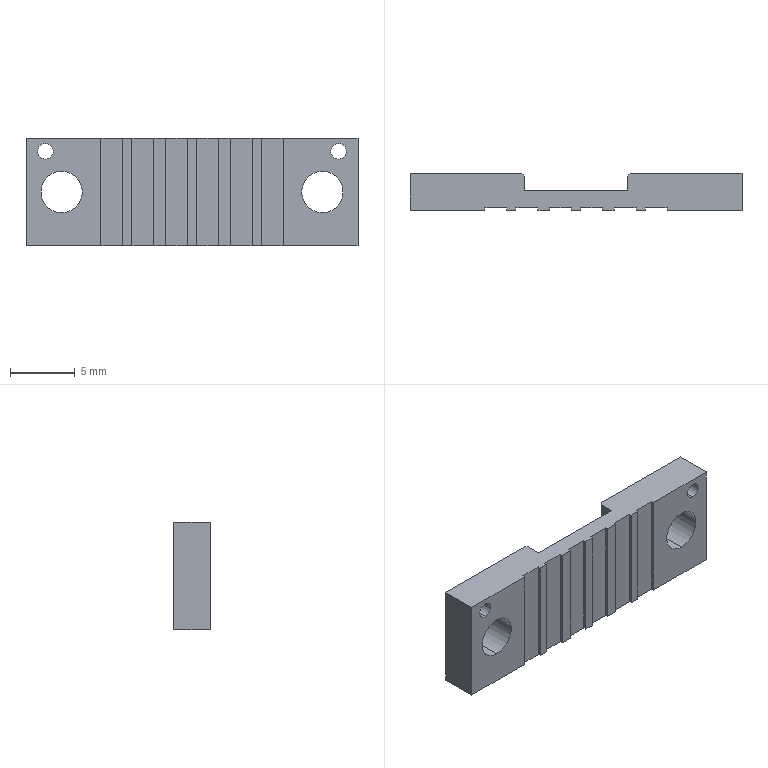Part | SolidWorks | features ICE 3, Chamfer 1, Extrusion 1 | 1 solid | 44 faces | box 25.7 x 2.85 x 8.3 mm | volume 448.741 mm3 | plane 36 | cylinder 8 | commonest cylinder face diameters 1.2 x4 3.2 x4
STEP:
#1=CARTESIAN_POINT('',(11.35,0.,2.55));
#2=VERTEX_POINT('',#1);
#3=CARTESIAN_POINT('',(11.35,0.,3.75));
#4=VERTEX_POINT('',#3);
#5=CARTESIAN_POINT('',(11.35,0.,3.15));
#6=DIRECTION('',(0.,1.,0.));
#7=DIRECTION('',(0.,0.,-1.));
#8=AXIS2_PLACEMENT_3D('',#5,#6,#7);
#9=CIRCLE('',#8,0.6);
#10=EDGE_CURVE('',#2,#4,#9,.T.);
#11=ORIENTED_EDGE('',*,*,#10,.F.);
#12=CARTESIAN_POINT('',(11.35,2.85,2.55));
#13=VERTEX_POINT('',#12);
#14=CARTESIAN_POINT('',(11.35,0.,2.55));
#15=DIRECTION('',(0.,1.,0.));
#16=VECTOR('',#15,1000.);
#17=LINE('',#14,#16);
#18=EDGE_CURVE('',#2,#13,#17,.T.);
#19=ORIENTED_EDGE('',*,*,#18,.T.);
#20=CARTESIAN_POINT('',(11.35,2.85,3.75));
#21=VERTEX_POINT('',#20);
#22=CARTESIAN_POINT('',(11.35,2.85,3.15));
#23=DIRECTION('',(0.,1.,0.));
#24=DIRECTION('',(0.,0.,-1.));
#25=AXIS2_PLACEMENT_3D('',#22,#23,#24);
#26=CIRCLE('',#25,0.6);
#27=EDGE_CURVE('',#13,#21,#26,.T.);
#28=ORIENTED_EDGE('',*,*,#27,.T.);
#29=CARTESIAN_POINT('',(11.35,0.,3.75));
#30=DIRECTION('',(0.,1.,0.));
#31=VECTOR('',#30,1000.);
#32=LINE('',#29,#31);
#33=EDGE_CURVE('',#4,#21,#32,.T.);
#34=ORIENTED_EDGE('',*,*,#33,.F.);
#35=EDGE_LOOP('',(#11,#19,#28,#34));
#36=FACE_OUTER_BOUND('',#35,.T.);
#37=CARTESIAN_POINT('',(11.35,0.,3.15));
#38=DIRECTION('',(0.,1.,0.));
#39=DIRECTION('',(0.,0.,1.));
#40=AXIS2_PLACEMENT_3D('',#37,#38,#39);
#41=CYLINDRICAL_SURFACE('',#40,0.6);
#42=ADVANCED_FACE('',(#36),#41,.F.);
#43=CARTESIAN_POINT('',(10.1,0.,-1.6));
#44=VERTEX_POINT('',#43);
#45=CARTESIAN_POINT('',(10.1,0.,1.6));
#46=VERTEX_POINT('',#45);
#47=CARTESIAN_POINT('',(10.1,0.,0.));
#48=DIRECTION('',(0.,1.,0.));
#49=DIRECTION('',(0.,0.,-1.));
#50=AXIS2_PLACEMENT_3D('',#47,#48,#49);
#51=CIRCLE('',#50,1.6);
#52=EDGE_CURVE('',#44,#46,#51,.T.);
#53=ORIENTED_EDGE('',*,*,#52,.F.);
#54=CARTESIAN_POINT('',(10.1,2.85,-1.6));
#55=VERTEX_POINT('',#54);
#56=CARTESIAN_POINT('',(10.1,0.,-1.6));
#57=DIRECTION('',(0.,1.,0.));
#58=VECTOR('',#57,1000.);
#59=LINE('',#56,#58);
#60=EDGE_CURVE('',#44,#55,#59,.T.);
#61=ORIENTED_EDGE('',*,*,#60,.T.);
#62=CARTESIAN_POINT('',(10.1,2.85,1.6));
#63=VERTEX_POINT('',#62);
#64=CARTESIAN_POINT('',(10.1,2.85,0.));
#65=DIRECTION('',(0.,1.,0.));
#66=DIRECTION('',(0.,0.,-1.));
#67=AXIS2_PLACEMENT_3D('',#64,#65,#66);
#68=CIRCLE('',#67,1.6);
#69=EDGE_CURVE('',#55,#63,#68,.T.);
#70=ORIENTED_EDGE('',*,*,#69,.T.);
#71=CARTESIAN_POINT('',(10.1,0.,1.6));
#72=DIRECTION('',(0.,1.,0.));
#73=VECTOR('',#72,1000.);
#74=LINE('',#71,#73);
#75=EDGE_CURVE('',#46,#63,#74,.T.);
#76=ORIENTED_EDGE('',*,*,#75,.F.);
#77=EDGE_LOOP('',(#53,#61,#70,#76));
#78=FACE_OUTER_BOUND('',#77,.T.);
#79=CARTESIAN_POINT('',(10.1,0.,0.));
#80=DIRECTION('',(0.,1.,0.));
#81=DIRECTION('',(0.,0.,1.));
#82=AXIS2_PLACEMENT_3D('',#79,#80,#81);
#83=CYLINDRICAL_SURFACE('',#82,1.6);
#84=ADVANCED_FACE('',(#78),#83,.F.);
#85=CARTESIAN_POINT('',(-11.35,0.,2.55));
#86=VERTEX_POINT('',#85);
#87=CARTESIAN_POINT('',(-11.35,0.,3.75));
#88=VERTEX_POINT('',#87);
#89=CARTESIAN_POINT('',(-11.35,0.,3.15));
#90=DIRECTION('',(0.,1.,0.));
#91=DIRECTION('',(0.,0.,1.));
#92=AXIS2_PLACEMENT_3D('',#89,#90,#91);
#93=CIRCLE('',#92,0.6);
#94=EDGE_CURVE('',#86,#88,#93,.T.);
#95=ORIENTED_EDGE('',*,*,#94,.F.);
#96=CARTESIAN_POINT('',(-11.35,2.85,2.55));
#97=VERTEX_POINT('',#96);
#98=CARTESIAN_POINT('',(-11.35,0.,2.55));
#99=DIRECTION('',(0.,1.,0.));
#100=VECTOR('',#99,1000.);
#101=LINE('',#98,#100);
#102=EDGE_CURVE('',#86,#97,#101,.T.);
#103=ORIENTED_EDGE('',*,*,#102,.T.);
#104=CARTESIAN_POINT('',(-11.35,2.85,3.75));
#105=VERTEX_POINT('',#104);
#106=CARTESIAN_POINT('',(-11.35,2.85,3.15));
#107=DIRECTION('',(0.,1.,0.));
#108=DIRECTION('',(0.,0.,1.));
#109=AXIS2_PLACEMENT_3D('',#106,#107,#108);
#110=CIRCLE('',#109,0.6);
#111=EDGE_CURVE('',#97,#105,#110,.T.);
#112=ORIENTED_EDGE('',*,*,#111,.T.);
#113=CARTESIAN_POINT('',(-11.35,0.,3.75));
#114=DIRECTION('',(0.,1.,0.));
#115=VECTOR('',#114,1000.);
#116=LINE('',#113,#115);
#117=EDGE_CURVE('',#88,#105,#116,.T.);
#118=ORIENTED_EDGE('',*,*,#117,.F.);
#119=EDGE_LOOP('',(#95,#103,#112,#118));
#120=FACE_OUTER_BOUND('',#119,.T.);
#121=CARTESIAN_POINT('',(-11.35,0.,3.15));
#122=DIRECTION('',(0.,1.,0.));
#123=DIRECTION('',(0.,0.,1.));
#124=AXIS2_PLACEMENT_3D('',#121,#122,#123);
#125=CYLINDRICAL_SURFACE('',#124,0.6);
#126=ADVANCED_FACE('',(#120),#125,.F.);
#127=CARTESIAN_POINT('',(-10.1,0.,-1.6));
#128=VERTEX_POINT('',#127);
#129=CARTESIAN_POINT('',(-10.1,0.,1.6));
#130=VERTEX_POINT('',#129);
#131=CARTESIAN_POINT('',(-10.1,0.,0.));
#132=DIRECTION('',(0.,1.,0.));
#133=DIRECTION('',(0.,0.,1.));
#134=AXIS2_PLACEMENT_3D('',#131,#132,#133);
#135=CIRCLE('',#134,1.6);
#136=EDGE_CURVE('',#128,#130,#135,.T.);
#137=ORIENTED_EDGE('',*,*,#136,.F.);
#138=CARTESIAN_POINT('',(-10.1,2.85,-1.6));
#139=VERTEX_POINT('',#138);
#140=CARTESIAN_POINT('',(-10.1,0.,-1.6));
#141=DIRECTION('',(0.,1.,0.));
#142=VECTOR('',#141,1000.);
#143=LINE('',#140,#142);
#144=EDGE_CURVE('',#128,#139,#143,.T.);
#145=ORIENTED_EDGE('',*,*,#144,.T.);
#146=CARTESIAN_POINT('',(-10.1,2.85,1.6));
#147=VERTEX_POINT('',#146);
#148=CARTESIAN_POINT('',(-10.1,2.85,0.));
#149=DIRECTION('',(0.,1.,0.));
#150=DIRECTION('',(0.,0.,1.));
#151=AXIS2_PLACEMENT_3D('',#148,#149,#150);
#152=CIRCLE('',#151,1.6);
#153=EDGE_CURVE('',#139,#147,#152,.T.);
#154=ORIENTED_EDGE('',*,*,#153,.T.);
#155=CARTESIAN_POINT('',(-10.1,0.,1.6));
#156=DIRECTION('',(0.,1.,0.));
#157=VECTOR('',#156,1000.);
#158=LINE('',#155,#157);
#159=EDGE_CURVE('',#130,#147,#158,.T.);
#160=ORIENTED_EDGE('',*,*,#159,.F.);
#161=EDGE_LOOP('',(#137,#145,#154,#160));
#162=FACE_OUTER_BOUND('',#161,.T.);
#163=CARTESIAN_POINT('',(-10.1,0.,0.));
#164=DIRECTION('',(0.,1.,0.));
#165=DIRECTION('',(0.,0.,1.));
#166=AXIS2_PLACEMENT_3D('',#163,#164,#165);
#167=CYLINDRICAL_SURFACE('',#166,1.6);
#168=ADVANCED_FACE('',(#162),#167,.F.);
#169=CARTESIAN_POINT('',(12.85,2.85,-4.15));
#170=VERTEX_POINT('',#169);
#171=CARTESIAN_POINT('',(4.2,2.85,-4.15));
#172=VERTEX_POINT('',#171);
#173=CARTESIAN_POINT('',(-12.85,2.85,-4.15));
#174=DIRECTION('',(-1.,0.,0.));
#175=VECTOR('',#174,1000.);
#176=LINE('',#173,#175);
#177=EDGE_CURVE('',#170,#172,#176,.T.);
#178=ORIENTED_EDGE('',*,*,#177,.T.);
#179=CARTESIAN_POINT('',(4.2,2.85,4.15));
#180=VERTEX_POINT('',#179);
#181=CARTESIAN_POINT('',(4.2,2.85,4.15));
#182=DIRECTION('',(0.,0.,1.));
#183=VECTOR('',#182,1000.);
#184=LINE('',#181,#183);
#185=EDGE_CURVE('',#172,#180,#184,.T.);
#186=ORIENTED_EDGE('',*,*,#185,.T.);
#187=CARTESIAN_POINT('',(12.85,2.85,4.15));
#188=VERTEX_POINT('',#187);
#189=CARTESIAN_POINT('',(-12.85,2.85,4.15));
#190=DIRECTION('',(1.,0.,0.));
#191=VECTOR('',#190,1000.);
#192=LINE('',#189,#191);
#193=EDGE_CURVE('',#180,#188,#192,.T.);
#194=ORIENTED_EDGE('',*,*,#193,.T.);
#195=CARTESIAN_POINT('',(12.85,2.85,-4.15));
#196=DIRECTION('',(0.,0.,-1.));
#197=VECTOR('',#196,1000.);
#198=LINE('',#195,#197);
#199=EDGE_CURVE('',#188,#170,#198,.T.);
#200=ORIENTED_EDGE('',*,*,#199,.T.);
#201=EDGE_LOOP('',(#178,#186,#194,#200));
#202=FACE_OUTER_BOUND('',#201,.T.);
#203=CARTESIAN_POINT('',(10.1,2.85,0.));
#204=DIRECTION('',(0.,1.,0.));
#205=DIRECTION('',(0.,0.,-1.));
#206=AXIS2_PLACEMENT_3D('',#203,#204,#205);
#207=CIRCLE('',#206,1.6);
#208=EDGE_CURVE('',#63,#55,#207,.T.);
#209=ORIENTED_EDGE('',*,*,#208,.F.);
#210=ORIENTED_EDGE('',*,*,#69,.F.);
#211=EDGE_LOOP('',(#209,#210));
#212=FACE_BOUND('',#211,.T.);
#213=CARTESIAN_POINT('',(11.35,2.85,3.15));
#214=DIRECTION('',(0.,1.,0.));
#215=DIRECTION('',(0.,0.,-1.));
#216=AXIS2_PLACEMENT_3D('',#213,#214,#215);
#217=CIRCLE('',#216,0.6);
#218=EDGE_CURVE('',#21,#13,#217,.T.);
#219=ORIENTED_EDGE('',*,*,#218,.F.);
#220=ORIENTED_EDGE('',*,*,#27,.F.);
#221=EDGE_LOOP('',(#219,#220));
#222=FACE_BOUND('',#221,.T.);
#223=CARTESIAN_POINT('',(0.,2.85,0.));
#224=DIRECTION('',(0.,1.,0.));
#225=DIRECTION('',(0.,0.,1.));
#226=AXIS2_PLACEMENT_3D('',#223,#224,#225);
#227=PLANE('',#226);
#228=ADVANCED_FACE('',(#202,#212,#222),#227,.T.);
#229=CARTESIAN_POINT('',(10.1,0.,0.));
#230=DIRECTION('',(0.,1.,0.));
#231=DIRECTION('',(0.,0.,-1.));
#232=AXIS2_PLACEMENT_3D('',#229,#230,#231);
#233=CIRCLE('',#232,1.6);
#234=EDGE_CURVE('',#46,#44,#233,.T.);
#235=ORIENTED_EDGE('',*,*,#234,.T.);
#236=ORIENTED_EDGE('',*,*,#52,.T.);
#237=EDGE_LOOP('',(#235,#236));
#238=FACE_BOUND('',#237,.T.);
#239=CARTESIAN_POINT('',(11.35,0.,3.15));
#240=DIRECTION('',(0.,1.,0.));
#241=DIRECTION('',(0.,0.,-1.));
#242=AXIS2_PLACEMENT_3D('',#239,#240,#241);
#243=CIRCLE('',#242,0.6);
#244=EDGE_CURVE('',#4,#2,#243,.T.);
#245=ORIENTED_EDGE('',*,*,#244,.T.);
#246=ORIENTED_EDGE('',*,*,#10,.T.);
#247=EDGE_LOOP('',(#245,#246));
#248=FACE_BOUND('',#247,.T.);
#249=CARTESIAN_POINT('',(7.05,0.,4.15));
#250=VERTEX_POINT('',#249);
#251=CARTESIAN_POINT('',(12.85,0.,4.15));
#252=VERTEX_POINT('',#251);
#253=CARTESIAN_POINT('',(-12.85,0.,4.15));
#254=DIRECTION('',(1.,0.,0.));
#255=VECTOR('',#254,1000.);
#256=LINE('',#253,#255);
#257=EDGE_CURVE('',#250,#252,#256,.T.);
#258=ORIENTED_EDGE('',*,*,#257,.F.);
#259=CARTESIAN_POINT('',(7.05,0.,-4.15));
#260=VERTEX_POINT('',#259);
#261=CARTESIAN_POINT('',(7.05,0.,4.15));
#262=DIRECTION('',(0.,0.,1.));
#263=VECTOR('',#262,1000.);
#264=LINE('',#261,#263);
#265=EDGE_CURVE('',#260,#250,#264,.T.);
#266=ORIENTED_EDGE('',*,*,#265,.F.);
#267=CARTESIAN_POINT('',(12.85,0.,-4.15));
#268=VERTEX_POINT('',#267);
#269=CARTESIAN_POINT('',(-12.85,0.,-4.15));
#270=DIRECTION('',(-1.,0.,0.));
#271=VECTOR('',#270,1000.);
#272=LINE('',#269,#271);
#273=EDGE_CURVE('',#268,#260,#272,.T.);
#274=ORIENTED_EDGE('',*,*,#273,.F.);
#275=CARTESIAN_POINT('',(12.85,0.,-4.15));
#276=DIRECTION('',(0.,0.,-1.));
#277=VECTOR('',#276,1000.);
#278=LINE('',#275,#277);
#279=EDGE_CURVE('',#252,#268,#278,.T.);
#280=ORIENTED_EDGE('',*,*,#279,.F.);
#281=EDGE_LOOP('',(#258,#266,#274,#280));
#282=FACE_OUTER_BOUND('',#281,.T.);
#283=CARTESIAN_POINT('',(0.,0.,0.));
#284=DIRECTION('',(0.,1.,0.));
#285=DIRECTION('',(0.,0.,1.));
#286=AXIS2_PLACEMENT_3D('',#283,#284,#285);
#287=PLANE('',#286);
#288=ADVANCED_FACE('',(#238,#248,#282),#287,.F.);
#289=CARTESIAN_POINT('',(5.35,0.,-4.15));
#290=VERTEX_POINT('',#289);
#291=CARTESIAN_POINT('',(4.65,0.,-4.15));
#292=VERTEX_POINT('',#291);
#293=CARTESIAN_POINT('',(-12.85,0.,-4.15));
#294=DIRECTION('',(-1.,0.,0.));
#295=VECTOR('',#294,1000.);
#296=LINE('',#293,#295);
#297=EDGE_CURVE('',#290,#292,#296,.T.);
#298=ORIENTED_EDGE('',*,*,#297,.F.);
#299=CARTESIAN_POINT('',(5.35,0.,4.15));
#300=VERTEX_POINT('',#299);
#301=CARTESIAN_POINT('',(5.35,0.,4.15));
#302=DIRECTION('',(0.,0.,-1.));
#303=VECTOR('',#302,1000.);
#304=LINE('',#301,#303);
#305=EDGE_CURVE('',#300,#290,#304,.T.);
#306=ORIENTED_EDGE('',*,*,#305,.F.);
#307=CARTESIAN_POINT('',(4.65,0.,4.15));
#308=VERTEX_POINT('',#307);
#309=CARTESIAN_POINT('',(-12.85,0.,4.15));
#310=DIRECTION('',(1.,0.,0.));
#311=VECTOR('',#310,1000.);
#312=LINE('',#309,#311);
#313=EDGE_CURVE('',#308,#300,#312,.T.);
#314=ORIENTED_EDGE('',*,*,#313,.F.);
#315=CARTESIAN_POINT('',(4.65,0.,4.15));
#316=DIRECTION('',(0.,0.,1.));
#317=VECTOR('',#316,1000.);
#318=LINE('',#315,#317);
#319=EDGE_CURVE('',#292,#308,#318,.T.);
#320=ORIENTED_EDGE('',*,*,#319,.F.);
#321=EDGE_LOOP('',(#298,#306,#314,#320));
#322=FACE_OUTER_BOUND('',#321,.T.);
#323=CARTESIAN_POINT('',(0.,0.,0.));
#324=DIRECTION('',(0.,1.,0.));
#325=DIRECTION('',(0.,0.,1.));
#326=AXIS2_PLACEMENT_3D('',#323,#324,#325);
#327=PLANE('',#326);
#328=ADVANCED_FACE('',(#322),#327,.F.);
#329=CARTESIAN_POINT('',(2.95,0.,-4.15));
#330=VERTEX_POINT('',#329);
#331=CARTESIAN_POINT('',(2.05,0.,-4.15));
#332=VERTEX_POINT('',#331);
#333=CARTESIAN_POINT('',(-12.85,0.,-4.15));
#334=DIRECTION('',(-1.,0.,0.));
#335=VECTOR('',#334,1000.);
#336=LINE('',#333,#335);
#337=EDGE_CURVE('',#330,#332,#336,.T.);
#338=ORIENTED_EDGE('',*,*,#337,.F.);
#339=CARTESIAN_POINT('',(2.95,0.,4.15));
#340=VERTEX_POINT('',#339);
#341=CARTESIAN_POINT('',(2.95,0.,4.15));
#342=DIRECTION('',(0.,0.,-1.));
#343=VECTOR('',#342,1000.);
#344=LINE('',#341,#343);
#345=EDGE_CURVE('',#340,#330,#344,.T.);
#346=ORIENTED_EDGE('',*,*,#345,.F.);
#347=CARTESIAN_POINT('',(2.05,0.,4.15));
#348=VERTEX_POINT('',#347);
#349=CARTESIAN_POINT('',(-12.85,0.,4.15));
#350=DIRECTION('',(1.,0.,0.));
#351=VECTOR('',#350,1000.);
#352=LINE('',#349,#351);
#353=EDGE_CURVE('',#348,#340,#352,.T.);
#354=ORIENTED_EDGE('',*,*,#353,.F.);
#355=CARTESIAN_POINT('',(2.05,0.,4.15));
#356=DIRECTION('',(0.,0.,1.));
#357=VECTOR('',#356,1000.);
#358=LINE('',#355,#357);
#359=EDGE_CURVE('',#332,#348,#358,.T.);
#360=ORIENTED_EDGE('',*,*,#359,.F.);
#361=EDGE_LOOP('',(#338,#346,#354,#360));
#362=FACE_OUTER_BOUND('',#361,.T.);
#363=CARTESIAN_POINT('',(0.,0.,0.));
#364=DIRECTION('',(0.,1.,0.));
#365=DIRECTION('',(0.,0.,1.));
#366=AXIS2_PLACEMENT_3D('',#363,#364,#365);
#367=PLANE('',#366);
#368=ADVANCED_FACE('',(#362),#367,.F.);
#369=CARTESIAN_POINT('',(-2.05,0.,-4.15));
#370=VERTEX_POINT('',#369);
#371=CARTESIAN_POINT('',(-2.95,0.,-4.15));
#372=VERTEX_POINT('',#371);
#373=CARTESIAN_POINT('',(-12.85,0.,-4.15));
#374=DIRECTION('',(-1.,0.,0.));
#375=VECTOR('',#374,1000.);
#376=LINE('',#373,#375);
#377=EDGE_CURVE('',#370,#372,#376,.T.);
#378=ORIENTED_EDGE('',*,*,#377,.F.);
#379=CARTESIAN_POINT('',(-2.05,0.,4.15));
#380=VERTEX_POINT('',#379);
#381=CARTESIAN_POINT('',(-2.05,0.,4.15));
#382=DIRECTION('',(0.,0.,-1.));
#383=VECTOR('',#382,1000.);
#384=LINE('',#381,#383);
#385=EDGE_CURVE('',#380,#370,#384,.T.);
#386=ORIENTED_EDGE('',*,*,#385,.F.);
#387=CARTESIAN_POINT('',(-2.95,0.,4.15));
#388=VERTEX_POINT('',#387);
#389=CARTESIAN_POINT('',(-12.85,0.,4.15));
#390=DIRECTION('',(1.,0.,0.));
#391=VECTOR('',#390,1000.);
#392=LINE('',#389,#391);
#393=EDGE_CURVE('',#388,#380,#392,.T.);
#394=ORIENTED_EDGE('',*,*,#393,.F.);
#395=CARTESIAN_POINT('',(-2.95,0.,4.15));
#396=DIRECTION('',(0.,0.,1.));
#397=VECTOR('',#396,1000.);
#398=LINE('',#395,#397);
#399=EDGE_CURVE('',#372,#388,#398,.T.);
#400=ORIENTED_EDGE('',*,*,#399,.F.);
#401=EDGE_LOOP('',(#378,#386,#394,#400));
#402=FACE_OUTER_BOUND('',#401,.T.);
#403=CARTESIAN_POINT('',(0.,0.,0.));
#404=DIRECTION('',(0.,1.,0.));
#405=DIRECTION('',(0.,0.,1.));
#406=AXIS2_PLACEMENT_3D('',#403,#404,#405);
#407=PLANE('',#406);
#408=ADVANCED_FACE('',(#402),#407,.F.);
#409=CARTESIAN_POINT('',(-4.65,0.,-4.15));
#410=VERTEX_POINT('',#409);
#411=CARTESIAN_POINT('',(-5.35,0.,-4.15));
#412=VERTEX_POINT('',#411);
#413=CARTESIAN_POINT('',(-12.85,0.,-4.15));
#414=DIRECTION('',(-1.,0.,0.));
#415=VECTOR('',#414,1000.);
#416=LINE('',#413,#415);
#417=EDGE_CURVE('',#410,#412,#416,.T.);
#418=ORIENTED_EDGE('',*,*,#417,.F.);
#419=CARTESIAN_POINT('',(-4.65,0.,4.15));
#420=VERTEX_POINT('',#419);
#421=CARTESIAN_POINT('',(-4.65,0.,4.15));
#422=DIRECTION('',(0.,0.,-1.));
#423=VECTOR('',#422,1000.);
#424=LINE('',#421,#423);
#425=EDGE_CURVE('',#420,#410,#424,.T.);
#426=ORIENTED_EDGE('',*,*,#425,.F.);
#427=CARTESIAN_POINT('',(-5.35,0.,4.15));
#428=VERTEX_POINT('',#427);
#429=CARTESIAN_POINT('',(-12.85,0.,4.15));
#430=DIRECTION('',(1.,0.,0.));
#431=VECTOR('',#430,1000.);
#432=LINE('',#429,#431);
#433=EDGE_CURVE('',#428,#420,#432,.T.);
#434=ORIENTED_EDGE('',*,*,#433,.F.);
#435=CARTESIAN_POINT('',(-5.35,0.,4.15));
#436=DIRECTION('',(0.,0.,1.));
#437=VECTOR('',#436,1000.);
#438=LINE('',#435,#437);
#439=EDGE_CURVE('',#412,#428,#438,.T.);
#440=ORIENTED_EDGE('',*,*,#439,.F.);
#441=EDGE_LOOP('',(#418,#426,#434,#440));
#442=FACE_OUTER_BOUND('',#441,.T.);
#443=CARTESIAN_POINT('',(0.,0.,0.));
#444=DIRECTION('',(0.,1.,0.));
#445=DIRECTION('',(0.,0.,1.));
#446=AXIS2_PLACEMENT_3D('',#443,#444,#445);
#447=PLANE('',#446);
#448=ADVANCED_FACE('',(#442),#447,.F.);
#449=CARTESIAN_POINT('',(-10.1,0.,0.));
#450=DIRECTION('',(0.,1.,0.));
#451=DIRECTION('',(0.,0.,1.));
#452=AXIS2_PLACEMENT_3D('',#449,#450,#451);
#453=CIRCLE('',#452,1.6);
#454=EDGE_CURVE('',#130,#128,#453,.T.);
#455=ORIENTED_EDGE('',*,*,#454,.T.);
#456=ORIENTED_EDGE('',*,*,#136,.T.);
#457=EDGE_LOOP('',(#455,#456));
#458=FACE_BOUND('',#457,.T.);
#459=CARTESIAN_POINT('',(-11.35,0.,3.15));
#460=DIRECTION('',(0.,1.,0.));
#461=DIRECTION('',(0.,0.,1.));
#462=AXIS2_PLACEMENT_3D('',#459,#460,#461);
#463=CIRCLE('',#462,0.6);
#464=EDGE_CURVE('',#88,#86,#463,.T.);
#465=ORIENTED_EDGE('',*,*,#464,.T.);
#466=ORIENTED_EDGE('',*,*,#94,.T.);
#467=EDGE_LOOP('',(#465,#466));
#468=FACE_BOUND('',#467,.T.);
#469=CARTESIAN_POINT('',(-7.05,0.,-4.15));
#470=VERTEX_POINT('',#469);
#471=CARTESIAN_POINT('',(-12.85,0.,-4.15));
#472=VERTEX_POINT('',#471);
#473=CARTESIAN_POINT('',(-12.85,0.,-4.15));
#474=DIRECTION('',(-1.,0.,0.));
#475=VECTOR('',#474,1000.);
#476=LINE('',#473,#475);
#477=EDGE_CURVE('',#470,#472,#476,.T.);
#478=ORIENTED_EDGE('',*,*,#477,.F.);
#479=CARTESIAN_POINT('',(-7.05,0.,4.15));
#480=VERTEX_POINT('',#479);
#481=CARTESIAN_POINT('',(-7.05,0.,4.15));
#482=DIRECTION('',(0.,0.,-1.));
#483=VECTOR('',#482,1000.);
#484=LINE('',#481,#483);
#485=EDGE_CURVE('',#480,#470,#484,.T.);
#486=ORIENTED_EDGE('',*,*,#485,.F.);
#487=CARTESIAN_POINT('',(-12.85,0.,4.15));
#488=VERTEX_POINT('',#487);
#489=CARTESIAN_POINT('',(-12.85,0.,4.15));
#490=DIRECTION('',(1.,0.,0.));
#491=VECTOR('',#490,1000.);
#492=LINE('',#489,#491);
#493=EDGE_CURVE('',#488,#480,#492,.T.);
#494=ORIENTED_EDGE('',*,*,#493,.F.);
#495=CARTESIAN_POINT('',(-12.85,0.,-4.15));
#496=DIRECTION('',(0.,0.,1.));
#497=VECTOR('',#496,1000.);
#498=LINE('',#495,#497);
#499=EDGE_CURVE('',#472,#488,#498,.T.);
#500=ORIENTED_EDGE('',*,*,#499,.F.);
#501=EDGE_LOOP('',(#478,#486,#494,#500));
#502=FACE_OUTER_BOUND('',#501,.T.);
#503=CARTESIAN_POINT('',(0.,0.,0.));
#504=DIRECTION('',(0.,1.,0.));
#505=DIRECTION('',(0.,0.,1.));
#506=AXIS2_PLACEMENT_3D('',#503,#504,#505);
#507=PLANE('',#506);
#508=ADVANCED_FACE('',(#458,#468,#502),#507,.F.);
#509=ORIENTED_EDGE('',*,*,#279,.T.);
#510=CARTESIAN_POINT('',(12.85,2.85,-4.15));
#511=DIRECTION('',(0.,-1.,0.));
#512=VECTOR('',#511,1000.);
#513=LINE('',#510,#512);
#514=EDGE_CURVE('',#170,#268,#513,.T.);
#515=ORIENTED_EDGE('',*,*,#514,.F.);
#516=ORIENTED_EDGE('',*,*,#199,.F.);
#517=CARTESIAN_POINT('',(12.85,2.85,4.15));
#518=DIRECTION('',(0.,-1.,0.));
#519=VECTOR('',#518,1000.);
#520=LINE('',#517,#519);
#521=EDGE_CURVE('',#188,#252,#520,.T.);
#522=ORIENTED_EDGE('',*,*,#521,.T.);
#523=EDGE_LOOP('',(#509,#515,#516,#522));
#524=FACE_OUTER_BOUND('',#523,.T.);
#525=CARTESIAN_POINT('',(12.85,2.85,-4.15));
#526=DIRECTION('',(-1.,0.,0.));
#527=DIRECTION('',(0.,0.,1.));
#528=AXIS2_PLACEMENT_3D('',#525,#526,#527);
#529=PLANE('',#528);
#530=ADVANCED_FACE('',(#524),#529,.F.);
#531=CARTESIAN_POINT('',(4.,1.5,-4.15));
#532=VERTEX_POINT('',#531);
#533=CARTESIAN_POINT('',(4.,2.65,-4.15));
#534=VERTEX_POINT('',#533);
#535=CARTESIAN_POINT('',(4.,1.5,-4.15));
#536=DIRECTION('',(0.,1.,0.));
#537=VECTOR('',#536,1000.);
#538=LINE('',#535,#537);
#539=EDGE_CURVE('',#532,#534,#538,.T.);
#540=ORIENTED_EDGE('',*,*,#539,.T.);
#541=CARTESIAN_POINT('',(4.,2.65,-4.15));
#542=DIRECTION('',(0.7071,0.7071,0.));
#543=VECTOR('',#542,1000.);
#544=LINE('',#541,#543);
#545=EDGE_CURVE('',#534,#172,#544,.T.);
#546=ORIENTED_EDGE('',*,*,#545,.T.);
#547=ORIENTED_EDGE('',*,*,#177,.F.);
#548=ORIENTED_EDGE('',*,*,#514,.T.);
#549=ORIENTED_EDGE('',*,*,#273,.T.);
#550=CARTESIAN_POINT('',(7.05,0.2,-4.15));
#551=VERTEX_POINT('',#550);
#552=CARTESIAN_POINT('',(7.05,0.2,-4.15));
#553=DIRECTION('',(0.,-1.,0.));
#554=VECTOR('',#553,1000.);
#555=LINE('',#552,#554);
#556=EDGE_CURVE('',#551,#260,#555,.T.);
#557=ORIENTED_EDGE('',*,*,#556,.F.);
#558=CARTESIAN_POINT('',(5.35,0.2,-4.15));
#559=VERTEX_POINT('',#558);
#560=CARTESIAN_POINT('',(7.05,0.2,-4.15));
#561=DIRECTION('',(1.,0.,0.));
#562=VECTOR('',#561,1000.);
#563=LINE('',#560,#562);
#564=EDGE_CURVE('',#559,#551,#563,.T.);
#565=ORIENTED_EDGE('',*,*,#564,.F.);
#566=CARTESIAN_POINT('',(5.35,0.2,-4.15));
#567=DIRECTION('',(0.,-1.,0.));
#568=VECTOR('',#567,1000.);
#569=LINE('',#566,#568);
#570=EDGE_CURVE('',#559,#290,#569,.T.);
#571=ORIENTED_EDGE('',*,*,#570,.T.);
#572=ORIENTED_EDGE('',*,*,#297,.T.);
#573=CARTESIAN_POINT('',(4.65,0.2,-4.15));
#574=VERTEX_POINT('',#573);
#575=CARTESIAN_POINT('',(4.65,0.2,-4.15));
#576=DIRECTION('',(0.,-1.,0.));
#577=VECTOR('',#576,1000.);
#578=LINE('',#575,#577);
#579=EDGE_CURVE('',#574,#292,#578,.T.);
#580=ORIENTED_EDGE('',*,*,#579,.F.);
#581=CARTESIAN_POINT('',(2.95,0.2,-4.15));
#582=VERTEX_POINT('',#581);
#583=CARTESIAN_POINT('',(4.65,0.2,-4.15));
#584=DIRECTION('',(1.,0.,0.));
#585=VECTOR('',#584,1000.);
#586=LINE('',#583,#585);
#587=EDGE_CURVE('',#582,#574,#586,.T.);
#588=ORIENTED_EDGE('',*,*,#587,.F.);
#589=CARTESIAN_POINT('',(2.95,0.2,-4.15));
#590=DIRECTION('',(0.,-1.,0.));
#591=VECTOR('',#590,1000.);
#592=LINE('',#589,#591);
#593=EDGE_CURVE('',#582,#330,#592,.T.);
#594=ORIENTED_EDGE('',*,*,#593,.T.);
#595=ORIENTED_EDGE('',*,*,#337,.T.);
#596=CARTESIAN_POINT('',(2.05,0.2,-4.15));
#597=VERTEX_POINT('',#596);
#598=CARTESIAN_POINT('',(2.05,0.2,-4.15));
#599=DIRECTION('',(0.,-1.,0.));
#600=VECTOR('',#599,1000.);
#601=LINE('',#598,#600);
#602=EDGE_CURVE('',#597,#332,#601,.T.);
#603=ORIENTED_EDGE('',*,*,#602,.F.);
#604=CARTESIAN_POINT('',(0.35,0.2,-4.15));
#605=VERTEX_POINT('',#604);
#606=CARTESIAN_POINT('',(2.05,0.2,-4.15));
#607=DIRECTION('',(1.,0.,0.));
#608=VECTOR('',#607,1000.);
#609=LINE('',#606,#608);
#610=EDGE_CURVE('',#605,#597,#609,.T.);
#611=ORIENTED_EDGE('',*,*,#610,.F.);
#612=CARTESIAN_POINT('',(0.35,0.,-4.15));
#613=VERTEX_POINT('',#612);
#614=CARTESIAN_POINT('',(0.35,0.2,-4.15));
#615=DIRECTION('',(0.,-1.,0.));
#616=VECTOR('',#615,1000.);
#617=LINE('',#614,#616);
#618=EDGE_CURVE('',#605,#613,#617,.T.);
#619=ORIENTED_EDGE('',*,*,#618,.T.);
#620=CARTESIAN_POINT('',(-0.35,0.,-4.15));
#621=VERTEX_POINT('',#620);
#622=CARTESIAN_POINT('',(-12.85,0.,-4.15));
#623=DIRECTION('',(-1.,0.,0.));
#624=VECTOR('',#623,1000.);
#625=LINE('',#622,#624);
#626=EDGE_CURVE('',#613,#621,#625,.T.);
#627=ORIENTED_EDGE('',*,*,#626,.T.);
#628=CARTESIAN_POINT('',(-0.35,0.2,-4.15));
#629=VERTEX_POINT('',#628);
#630=CARTESIAN_POINT('',(-0.35,0.2,-4.15));
#631=DIRECTION('',(0.,-1.,0.));
#632=VECTOR('',#631,1000.);
#633=LINE('',#630,#632);
#634=EDGE_CURVE('',#629,#621,#633,.T.);
#635=ORIENTED_EDGE('',*,*,#634,.F.);
#636=CARTESIAN_POINT('',(-2.05,0.2,-4.15));
#637=VERTEX_POINT('',#636);
#638=CARTESIAN_POINT('',(-2.05,0.2,-4.15));
#639=DIRECTION('',(1.,0.,0.));
#640=VECTOR('',#639,1000.);
#641=LINE('',#638,#640);
#642=EDGE_CURVE('',#637,#629,#641,.T.);
#643=ORIENTED_EDGE('',*,*,#642,.F.);
#644=CARTESIAN_POINT('',(-2.05,0.2,-4.15));
#645=DIRECTION('',(0.,-1.,0.));
#646=VECTOR('',#645,1000.);
#647=LINE('',#644,#646);
#648=EDGE_CURVE('',#637,#370,#647,.T.);
#649=ORIENTED_EDGE('',*,*,#648,.T.);
#650=ORIENTED_EDGE('',*,*,#377,.T.);
#651=CARTESIAN_POINT('',(-2.95,0.2,-4.15));
#652=VERTEX_POINT('',#651);
#653=CARTESIAN_POINT('',(-2.95,0.2,-4.15));
#654=DIRECTION('',(0.,-1.,0.));
#655=VECTOR('',#654,1000.);
#656=LINE('',#653,#655);
#657=EDGE_CURVE('',#652,#372,#656,.T.);
#658=ORIENTED_EDGE('',*,*,#657,.F.);
#659=CARTESIAN_POINT('',(-4.65,0.2,-4.15));
#660=VERTEX_POINT('',#659);
#661=CARTESIAN_POINT('',(-4.65,0.2,-4.15));
#662=DIRECTION('',(1.,0.,0.));
#663=VECTOR('',#662,1000.);
#664=LINE('',#661,#663);
#665=EDGE_CURVE('',#660,#652,#664,.T.);
#666=ORIENTED_EDGE('',*,*,#665,.F.);
#667=CARTESIAN_POINT('',(-4.65,0.2,-4.15));
#668=DIRECTION('',(0.,-1.,0.));
#669=VECTOR('',#668,1000.);
#670=LINE('',#667,#669);
#671=EDGE_CURVE('',#660,#410,#670,.T.);
#672=ORIENTED_EDGE('',*,*,#671,.T.);
#673=ORIENTED_EDGE('',*,*,#417,.T.);
#674=CARTESIAN_POINT('',(-5.35,0.2,-4.15));
#675=VERTEX_POINT('',#674);
#676=CARTESIAN_POINT('',(-5.35,0.2,-4.15));
#677=DIRECTION('',(0.,-1.,0.));
#678=VECTOR('',#677,1000.);
#679=LINE('',#676,#678);
#680=EDGE_CURVE('',#675,#412,#679,.T.);
#681=ORIENTED_EDGE('',*,*,#680,.F.);
#682=CARTESIAN_POINT('',(-7.05,0.2,-4.15));
#683=VERTEX_POINT('',#682);
#684=CARTESIAN_POINT('',(-7.05,0.2,-4.15));
#685=DIRECTION('',(1.,0.,0.));
#686=VECTOR('',#685,1000.);
#687=LINE('',#684,#686);
#688=EDGE_CURVE('',#683,#675,#687,.T.);
#689=ORIENTED_EDGE('',*,*,#688,.F.);
#690=CARTESIAN_POINT('',(-7.05,0.2,-4.15));
#691=DIRECTION('',(0.,-1.,0.));
#692=VECTOR('',#691,1000.);
#693=LINE('',#690,#692);
#694=EDGE_CURVE('',#683,#470,#693,.T.);
#695=ORIENTED_EDGE('',*,*,#694,.T.);
#696=ORIENTED_EDGE('',*,*,#477,.T.);
#697=CARTESIAN_POINT('',(-12.85,2.85,-4.15));
#698=VERTEX_POINT('',#697);
#699=CARTESIAN_POINT('',(-12.85,2.85,-4.15));
#700=DIRECTION('',(0.,-1.,0.));
#701=VECTOR('',#700,1000.);
#702=LINE('',#699,#701);
#703=EDGE_CURVE('',#698,#472,#702,.T.);
#704=ORIENTED_EDGE('',*,*,#703,.F.);
#705=CARTESIAN_POINT('',(-4.2,2.85,-4.15));
#706=VERTEX_POINT('',#705);
#707=CARTESIAN_POINT('',(-12.85,2.85,-4.15));
#708=DIRECTION('',(-1.,0.,0.));
#709=VECTOR('',#708,1000.);
#710=LINE('',#707,#709);
#711=EDGE_CURVE('',#706,#698,#710,.T.);
#712=ORIENTED_EDGE('',*,*,#711,.F.);
#713=CARTESIAN_POINT('',(-4.,2.65,-4.15));
#714=VERTEX_POINT('',#713);
#715=CARTESIAN_POINT('',(-4.,2.65,-4.15));
#716=DIRECTION('',(0.7071,-0.7071,0.));
#717=VECTOR('',#716,1000.);
#718=LINE('',#715,#717);
#719=EDGE_CURVE('',#706,#714,#718,.T.);
#720=ORIENTED_EDGE('',*,*,#719,.T.);
#721=CARTESIAN_POINT('',(-4.,1.5,-4.15));
#722=VERTEX_POINT('',#721);
#723=CARTESIAN_POINT('',(-4.,1.5,-4.15));
#724=DIRECTION('',(0.,1.,0.));
#725=VECTOR('',#724,1000.);
#726=LINE('',#723,#725);
#727=EDGE_CURVE('',#722,#714,#726,.T.);
#728=ORIENTED_EDGE('',*,*,#727,.F.);
#729=CARTESIAN_POINT('',(-4.,1.5,-4.15));
#730=DIRECTION('',(-1.,0.,0.));
#731=VECTOR('',#730,1000.);
#732=LINE('',#729,#731);
#733=EDGE_CURVE('',#532,#722,#732,.T.);
#734=ORIENTED_EDGE('',*,*,#733,.F.);
#735=EDGE_LOOP('',(#540,#546,#547,#548,#549,#557,#565,#571,#572,#580,#588,#594,#595,#603,#611,#619,#627,#635,#643,#649,#650,#658,#666,#672,#673,#681,#689,#695,#696,#704,#712,#720,#728,#734));
#736=FACE_OUTER_BOUND('',#735,.T.);
#737=CARTESIAN_POINT('',(-12.85,2.85,-4.15));
#738=DIRECTION('',(0.,0.,1.));
#739=DIRECTION('',(1.,0.,0.));
#740=AXIS2_PLACEMENT_3D('',#737,#738,#739);
#741=PLANE('',#740);
#742=ADVANCED_FACE('',(#736),#741,.F.);
#743=ORIENTED_EDGE('',*,*,#499,.T.);
#744=CARTESIAN_POINT('',(-12.85,2.85,4.15));
#745=VERTEX_POINT('',#744);
#746=CARTESIAN_POINT('',(-12.85,2.85,4.15));
#747=DIRECTION('',(0.,-1.,0.));
#748=VECTOR('',#747,1000.);
#749=LINE('',#746,#748);
#750=EDGE_CURVE('',#745,#488,#749,.T.);
#751=ORIENTED_EDGE('',*,*,#750,.F.);
#752=CARTESIAN_POINT('',(-12.85,2.85,-4.15));
#753=DIRECTION('',(0.,0.,1.));
#754=VECTOR('',#753,1000.);
#755=LINE('',#752,#754);
#756=EDGE_CURVE('',#698,#745,#755,.T.);
#757=ORIENTED_EDGE('',*,*,#756,.F.);
#758=ORIENTED_EDGE('',*,*,#703,.T.);
#759=EDGE_LOOP('',(#743,#751,#757,#758));
#760=FACE_OUTER_BOUND('',#759,.T.);
#761=CARTESIAN_POINT('',(-12.85,2.85,-4.15));
#762=DIRECTION('',(1.,0.,0.));
#763=DIRECTION('',(0.,0.,-1.));
#764=AXIS2_PLACEMENT_3D('',#761,#762,#763);
#765=PLANE('',#764);
#766=ADVANCED_FACE('',(#760),#765,.F.);
#767=ORIENTED_EDGE('',*,*,#193,.F.);
#768=CARTESIAN_POINT('',(4.,2.65,4.15));
#769=VERTEX_POINT('',#768);
#770=CARTESIAN_POINT('',(4.,2.65,4.15));
#771=DIRECTION('',(-0.7071,-0.7071,0.));
#772=VECTOR('',#771,1000.);
#773=LINE('',#770,#772);
#774=EDGE_CURVE('',#180,#769,#773,.T.);
#775=ORIENTED_EDGE('',*,*,#774,.T.);
#776=CARTESIAN_POINT('',(4.,1.5,4.15));
#777=VERTEX_POINT('',#776);
#778=CARTESIAN_POINT('',(4.,1.5,4.15));
#779=DIRECTION('',(0.,1.,0.));
#780=VECTOR('',#779,1000.);
#781=LINE('',#778,#780);
#782=EDGE_CURVE('',#777,#769,#781,.T.);
#783=ORIENTED_EDGE('',*,*,#782,.F.);
#784=CARTESIAN_POINT('',(-4.,1.5,4.15));
#785=VERTEX_POINT('',#784);
#786=CARTESIAN_POINT('',(-4.,1.5,4.15));
#787=DIRECTION('',(1.,0.,0.));
#788=VECTOR('',#787,1000.);
#789=LINE('',#786,#788);
#790=EDGE_CURVE('',#785,#777,#789,.T.);
#791=ORIENTED_EDGE('',*,*,#790,.F.);
#792=CARTESIAN_POINT('',(-4.,2.65,4.15));
#793=VERTEX_POINT('',#792);
#794=CARTESIAN_POINT('',(-4.,1.5,4.15));
#795=DIRECTION('',(0.,1.,0.));
#796=VECTOR('',#795,1000.);
#797=LINE('',#794,#796);
#798=EDGE_CURVE('',#785,#793,#797,.T.);
#799=ORIENTED_EDGE('',*,*,#798,.T.);
#800=CARTESIAN_POINT('',(-4.2,2.85,4.15));
#801=VERTEX_POINT('',#800);
#802=CARTESIAN_POINT('',(-4.,2.65,4.15));
#803=DIRECTION('',(-0.7071,0.7071,0.));
#804=VECTOR('',#803,1000.);
#805=LINE('',#802,#804);
#806=EDGE_CURVE('',#793,#801,#805,.T.);
#807=ORIENTED_EDGE('',*,*,#806,.T.);
#808=CARTESIAN_POINT('',(-12.85,2.85,4.15));
#809=DIRECTION('',(1.,0.,0.));
#810=VECTOR('',#809,1000.);
#811=LINE('',#808,#810);
#812=EDGE_CURVE('',#745,#801,#811,.T.);
#813=ORIENTED_EDGE('',*,*,#812,.F.);
#814=ORIENTED_EDGE('',*,*,#750,.T.);
#815=ORIENTED_EDGE('',*,*,#493,.T.);
#816=CARTESIAN_POINT('',(-7.05,0.2,4.15));
#817=VERTEX_POINT('',#816);
#818=CARTESIAN_POINT('',(-7.05,0.2,4.15));
#819=DIRECTION('',(0.,-1.,0.));
#820=VECTOR('',#819,1000.);
#821=LINE('',#818,#820);
#822=EDGE_CURVE('',#817,#480,#821,.T.);
#823=ORIENTED_EDGE('',*,*,#822,.F.);
#824=CARTESIAN_POINT('',(-5.35,0.2,4.15));
#825=VERTEX_POINT('',#824);
#826=CARTESIAN_POINT('',(-7.05,0.2,4.15));
#827=DIRECTION('',(-1.,0.,0.));
#828=VECTOR('',#827,1000.);
#829=LINE('',#826,#828);
#830=EDGE_CURVE('',#825,#817,#829,.T.);
#831=ORIENTED_EDGE('',*,*,#830,.F.);
#832=CARTESIAN_POINT('',(-5.35,0.2,4.15));
#833=DIRECTION('',(0.,-1.,0.));
#834=VECTOR('',#833,1000.);
#835=LINE('',#832,#834);
#836=EDGE_CURVE('',#825,#428,#835,.T.);
#837=ORIENTED_EDGE('',*,*,#836,.T.);
#838=ORIENTED_EDGE('',*,*,#433,.T.);
#839=CARTESIAN_POINT('',(-4.65,0.2,4.15));
#840=VERTEX_POINT('',#839);
#841=CARTESIAN_POINT('',(-4.65,0.2,4.15));
#842=DIRECTION('',(0.,-1.,0.));
#843=VECTOR('',#842,1000.);
#844=LINE('',#841,#843);
#845=EDGE_CURVE('',#840,#420,#844,.T.);
#846=ORIENTED_EDGE('',*,*,#845,.F.);
#847=CARTESIAN_POINT('',(-2.95,0.2,4.15));
#848=VERTEX_POINT('',#847);
#849=CARTESIAN_POINT('',(-4.65,0.2,4.15));
#850=DIRECTION('',(-1.,0.,0.));
#851=VECTOR('',#850,1000.);
#852=LINE('',#849,#851);
#853=EDGE_CURVE('',#848,#840,#852,.T.);
#854=ORIENTED_EDGE('',*,*,#853,.F.);
#855=CARTESIAN_POINT('',(-2.95,0.2,4.15));
#856=DIRECTION('',(0.,-1.,0.));
#857=VECTOR('',#856,1000.);
#858=LINE('',#855,#857);
#859=EDGE_CURVE('',#848,#388,#858,.T.);
#860=ORIENTED_EDGE('',*,*,#859,.T.);
#861=ORIENTED_EDGE('',*,*,#393,.T.);
#862=CARTESIAN_POINT('',(-2.05,0.2,4.15));
#863=VERTEX_POINT('',#862);
#864=CARTESIAN_POINT('',(-2.05,0.2,4.15));
#865=DIRECTION('',(0.,-1.,0.));
#866=VECTOR('',#865,1000.);
#867=LINE('',#864,#866);
#868=EDGE_CURVE('',#863,#380,#867,.T.);
#869=ORIENTED_EDGE('',*,*,#868,.F.);
#870=CARTESIAN_POINT('',(-0.35,0.2,4.15));
#871=VERTEX_POINT('',#870);
#872=CARTESIAN_POINT('',(-2.05,0.2,4.15));
#873=DIRECTION('',(-1.,0.,0.));
#874=VECTOR('',#873,1000.);
#875=LINE('',#872,#874);
#876=EDGE_CURVE('',#871,#863,#875,.T.);
#877=ORIENTED_EDGE('',*,*,#876,.F.);
#878=CARTESIAN_POINT('',(-0.35,0.,4.15));
#879=VERTEX_POINT('',#878);
#880=CARTESIAN_POINT('',(-0.35,0.2,4.15));
#881=DIRECTION('',(0.,-1.,0.));
#882=VECTOR('',#881,1000.);
#883=LINE('',#880,#882);
#884=EDGE_CURVE('',#871,#879,#883,.T.);
#885=ORIENTED_EDGE('',*,*,#884,.T.);
#886=CARTESIAN_POINT('',(0.35,0.,4.15));
#887=VERTEX_POINT('',#886);
#888=CARTESIAN_POINT('',(-12.85,0.,4.15));
#889=DIRECTION('',(1.,0.,0.));
#890=VECTOR('',#889,1000.);
#891=LINE('',#888,#890);
#892=EDGE_CURVE('',#879,#887,#891,.T.);
#893=ORIENTED_EDGE('',*,*,#892,.T.);
#894=CARTESIAN_POINT('',(0.35,0.2,4.15));
#895=VERTEX_POINT('',#894);
#896=CARTESIAN_POINT('',(0.35,0.2,4.15));
#897=DIRECTION('',(0.,-1.,0.));
#898=VECTOR('',#897,1000.);
#899=LINE('',#896,#898);
#900=EDGE_CURVE('',#895,#887,#899,.T.);
#901=ORIENTED_EDGE('',*,*,#900,.F.);
#902=CARTESIAN_POINT('',(2.05,0.2,4.15));
#903=VERTEX_POINT('',#902);
#904=CARTESIAN_POINT('',(2.05,0.2,4.15));
#905=DIRECTION('',(-1.,0.,0.));
#906=VECTOR('',#905,1000.);
#907=LINE('',#904,#906);
#908=EDGE_CURVE('',#903,#895,#907,.T.);
#909=ORIENTED_EDGE('',*,*,#908,.F.);
#910=CARTESIAN_POINT('',(2.05,0.2,4.15));
#911=DIRECTION('',(0.,-1.,0.));
#912=VECTOR('',#911,1000.);
#913=LINE('',#910,#912);
#914=EDGE_CURVE('',#903,#348,#913,.T.);
#915=ORIENTED_EDGE('',*,*,#914,.T.);
#916=ORIENTED_EDGE('',*,*,#353,.T.);
#917=CARTESIAN_POINT('',(2.95,0.2,4.15));
#918=VERTEX_POINT('',#917);
#919=CARTESIAN_POINT('',(2.95,0.2,4.15));
#920=DIRECTION('',(0.,-1.,0.));
#921=VECTOR('',#920,1000.);
#922=LINE('',#919,#921);
#923=EDGE_CURVE('',#918,#340,#922,.T.);
#924=ORIENTED_EDGE('',*,*,#923,.F.);
#925=CARTESIAN_POINT('',(4.65,0.2,4.15));
#926=VERTEX_POINT('',#925);
#927=CARTESIAN_POINT('',(4.65,0.2,4.15));
#928=DIRECTION('',(-1.,0.,0.));
#929=VECTOR('',#928,1000.);
#930=LINE('',#927,#929);
#931=EDGE_CURVE('',#926,#918,#930,.T.);
#932=ORIENTED_EDGE('',*,*,#931,.F.);
#933=CARTESIAN_POINT('',(4.65,0.2,4.15));
#934=DIRECTION('',(0.,-1.,0.));
#935=VECTOR('',#934,1000.);
#936=LINE('',#933,#935);
#937=EDGE_CURVE('',#926,#308,#936,.T.);
#938=ORIENTED_EDGE('',*,*,#937,.T.);
#939=ORIENTED_EDGE('',*,*,#313,.T.);
#940=CARTESIAN_POINT('',(5.35,0.2,4.15));
#941=VERTEX_POINT('',#940);
#942=CARTESIAN_POINT('',(5.35,0.2,4.15));
#943=DIRECTION('',(0.,-1.,0.));
#944=VECTOR('',#943,1000.);
#945=LINE('',#942,#944);
#946=EDGE_CURVE('',#941,#300,#945,.T.);
#947=ORIENTED_EDGE('',*,*,#946,.F.);
#948=CARTESIAN_POINT('',(7.05,0.2,4.15));
#949=VERTEX_POINT('',#948);
#950=CARTESIAN_POINT('',(7.05,0.2,4.15));
#951=DIRECTION('',(-1.,0.,0.));
#952=VECTOR('',#951,1000.);
#953=LINE('',#950,#952);
#954=EDGE_CURVE('',#949,#941,#953,.T.);
#955=ORIENTED_EDGE('',*,*,#954,.F.);
#956=CARTESIAN_POINT('',(7.05,0.2,4.15));
#957=DIRECTION('',(0.,-1.,0.));
#958=VECTOR('',#957,1000.);
#959=LINE('',#956,#958);
#960=EDGE_CURVE('',#949,#250,#959,.T.);
#961=ORIENTED_EDGE('',*,*,#960,.T.);
#962=ORIENTED_EDGE('',*,*,#257,.T.);
#963=ORIENTED_EDGE('',*,*,#521,.F.);
#964=EDGE_LOOP('',(#767,#775,#783,#791,#799,#807,#813,#814,#815,#823,#831,#837,#838,#846,#854,#860,#861,#869,#877,#885,#893,#901,#909,#915,#916,#924,#932,#938,#939,#947,#955,#961,#962,#963));
#965=FACE_OUTER_BOUND('',#964,.T.);
#966=CARTESIAN_POINT('',(-12.85,2.85,4.15));
#967=DIRECTION('',(0.,0.,-1.));
#968=DIRECTION('',(-1.,0.,0.));
#969=AXIS2_PLACEMENT_3D('',#966,#967,#968);
#970=PLANE('',#969);
#971=ADVANCED_FACE('',(#965),#970,.F.);
#972=ORIENTED_EDGE('',*,*,#812,.T.);
#973=CARTESIAN_POINT('',(-4.2,2.85,-4.15));
#974=DIRECTION('',(0.,0.,-1.));
#975=VECTOR('',#974,1000.);
#976=LINE('',#973,#975);
#977=EDGE_CURVE('',#801,#706,#976,.T.);
#978=ORIENTED_EDGE('',*,*,#977,.T.);
#979=ORIENTED_EDGE('',*,*,#711,.T.);
#980=ORIENTED_EDGE('',*,*,#756,.T.);
#981=EDGE_LOOP('',(#972,#978,#979,#980));
#982=FACE_OUTER_BOUND('',#981,.T.);
#983=CARTESIAN_POINT('',(-11.35,2.85,3.15));
#984=DIRECTION('',(0.,1.,0.));
#985=DIRECTION('',(0.,0.,1.));
#986=AXIS2_PLACEMENT_3D('',#983,#984,#985);
#987=CIRCLE('',#986,0.6);
#988=EDGE_CURVE('',#105,#97,#987,.T.);
#989=ORIENTED_EDGE('',*,*,#988,.F.);
#990=ORIENTED_EDGE('',*,*,#111,.F.);
#991=EDGE_LOOP('',(#989,#990));
#992=FACE_BOUND('',#991,.T.);
#993=CARTESIAN_POINT('',(-10.1,2.85,0.));
#994=DIRECTION('',(0.,1.,0.));
#995=DIRECTION('',(0.,0.,1.));
#996=AXIS2_PLACEMENT_3D('',#993,#994,#995);
#997=CIRCLE('',#996,1.6);
#998=EDGE_CURVE('',#147,#139,#997,.T.);
#999=ORIENTED_EDGE('',*,*,#998,.F.);
#1000=ORIENTED_EDGE('',*,*,#153,.F.);
#1001=EDGE_LOOP('',(#999,#1000));
#1002=FACE_BOUND('',#1001,.T.);
#1003=CARTESIAN_POINT('',(0.,2.85,0.));
#1004=DIRECTION('',(0.,1.,0.));
#1005=DIRECTION('',(0.,0.,1.));
#1006=AXIS2_PLACEMENT_3D('',#1003,#1004,#1005);
#1007=PLANE('',#1006);
#1008=ADVANCED_FACE('',(#982,#992,#1002),#1007,.T.);
#1009=ORIENTED_EDGE('',*,*,#626,.F.);
#1010=CARTESIAN_POINT('',(0.35,0.,4.15));
#1011=DIRECTION('',(0.,0.,-1.));
#1012=VECTOR('',#1011,1000.);
#1013=LINE('',#1010,#1012);
#1014=EDGE_CURVE('',#887,#613,#1013,.T.);
#1015=ORIENTED_EDGE('',*,*,#1014,.F.);
#1016=ORIENTED_EDGE('',*,*,#892,.F.);
#1017=CARTESIAN_POINT('',(-0.35,0.,4.15));
#1018=DIRECTION('',(0.,0.,1.));
#1019=VECTOR('',#1018,1000.);
#1020=LINE('',#1017,#1019);
#1021=EDGE_CURVE('',#621,#879,#1020,.T.);
#1022=ORIENTED_EDGE('',*,*,#1021,.F.);
#1023=EDGE_LOOP('',(#1009,#1015,#1016,#1022));
#1024=FACE_OUTER_BOUND('',#1023,.T.);
#1025=CARTESIAN_POINT('',(0.,0.,0.));
#1026=DIRECTION('',(0.,1.,0.));
#1027=DIRECTION('',(0.,0.,1.));
#1028=AXIS2_PLACEMENT_3D('',#1025,#1026,#1027);
#1029=PLANE('',#1028);
#1030=ADVANCED_FACE('',(#1024),#1029,.F.);
#1031=ORIENTED_EDGE('',*,*,#144,.F.);
#1032=ORIENTED_EDGE('',*,*,#454,.F.);
#1033=ORIENTED_EDGE('',*,*,#159,.T.);
#1034=ORIENTED_EDGE('',*,*,#998,.T.);
#1035=EDGE_LOOP('',(#1031,#1032,#1033,#1034));
#1036=FACE_OUTER_BOUND('',#1035,.T.);
#1037=CARTESIAN_POINT('',(-10.1,0.,0.));
#1038=DIRECTION('',(0.,1.,0.));
#1039=DIRECTION('',(0.,0.,1.));
#1040=AXIS2_PLACEMENT_3D('',#1037,#1038,#1039);
#1041=CYLINDRICAL_SURFACE('',#1040,1.6);
#1042=ADVANCED_FACE('',(#1036),#1041,.F.);
#1043=ORIENTED_EDGE('',*,*,#102,.F.);
#1044=ORIENTED_EDGE('',*,*,#464,.F.);
#1045=ORIENTED_EDGE('',*,*,#117,.T.);
#1046=ORIENTED_EDGE('',*,*,#988,.T.);
#1047=EDGE_LOOP('',(#1043,#1044,#1045,#1046));
#1048=FACE_OUTER_BOUND('',#1047,.T.);
#1049=CARTESIAN_POINT('',(-11.35,0.,3.15));
#1050=DIRECTION('',(0.,1.,0.));
#1051=DIRECTION('',(0.,0.,1.));
#1052=AXIS2_PLACEMENT_3D('',#1049,#1050,#1051);
#1053=CYLINDRICAL_SURFACE('',#1052,0.6);
#1054=ADVANCED_FACE('',(#1048),#1053,.F.);
#1055=ORIENTED_EDGE('',*,*,#60,.F.);
#1056=ORIENTED_EDGE('',*,*,#234,.F.);
#1057=ORIENTED_EDGE('',*,*,#75,.T.);
#1058=ORIENTED_EDGE('',*,*,#208,.T.);
#1059=EDGE_LOOP('',(#1055,#1056,#1057,#1058));
#1060=FACE_OUTER_BOUND('',#1059,.T.);
#1061=CARTESIAN_POINT('',(10.1,0.,0.));
#1062=DIRECTION('',(0.,1.,0.));
#1063=DIRECTION('',(0.,0.,1.));
#1064=AXIS2_PLACEMENT_3D('',#1061,#1062,#1063);
#1065=CYLINDRICAL_SURFACE('',#1064,1.6);
#1066=ADVANCED_FACE('',(#1060),#1065,.F.);
#1067=ORIENTED_EDGE('',*,*,#18,.F.);
#1068=ORIENTED_EDGE('',*,*,#244,.F.);
#1069=ORIENTED_EDGE('',*,*,#33,.T.);
#1070=ORIENTED_EDGE('',*,*,#218,.T.);
#1071=EDGE_LOOP('',(#1067,#1068,#1069,#1070));
#1072=FACE_OUTER_BOUND('',#1071,.T.);
#1073=CARTESIAN_POINT('',(11.35,0.,3.15));
#1074=DIRECTION('',(0.,1.,0.));
#1075=DIRECTION('',(0.,0.,1.));
#1076=AXIS2_PLACEMENT_3D('',#1073,#1074,#1075);
#1077=CYLINDRICAL_SURFACE('',#1076,0.6);
#1078=ADVANCED_FACE('',(#1072),#1077,.F.);
#1079=ORIENTED_EDGE('',*,*,#485,.T.);
#1080=ORIENTED_EDGE('',*,*,#694,.F.);
#1081=CARTESIAN_POINT('',(-7.05,0.2,4.15));
#1082=DIRECTION('',(0.,0.,-1.));
#1083=VECTOR('',#1082,1000.);
#1084=LINE('',#1081,#1083);
#1085=EDGE_CURVE('',#817,#683,#1084,.T.);
#1086=ORIENTED_EDGE('',*,*,#1085,.F.);
#1087=ORIENTED_EDGE('',*,*,#822,.T.);
#1088=EDGE_LOOP('',(#1079,#1080,#1086,#1087));
#1089=FACE_OUTER_BOUND('',#1088,.T.);
#1090=CARTESIAN_POINT('',(-7.05,0.2,4.15));
#1091=DIRECTION('',(-1.,0.,0.));
#1092=DIRECTION('',(0.,0.,1.));
#1093=AXIS2_PLACEMENT_3D('',#1090,#1091,#1092);
#1094=PLANE('',#1093);
#1095=ADVANCED_FACE('',(#1089),#1094,.F.);
#1096=ORIENTED_EDGE('',*,*,#439,.T.);
#1097=ORIENTED_EDGE('',*,*,#836,.F.);
#1098=CARTESIAN_POINT('',(-5.35,0.2,4.15));
#1099=DIRECTION('',(0.,0.,1.));
#1100=VECTOR('',#1099,1000.);
#1101=LINE('',#1098,#1100);
#1102=EDGE_CURVE('',#675,#825,#1101,.T.);
#1103=ORIENTED_EDGE('',*,*,#1102,.F.);
#1104=ORIENTED_EDGE('',*,*,#680,.T.);
#1105=EDGE_LOOP('',(#1096,#1097,#1103,#1104));
#1106=FACE_OUTER_BOUND('',#1105,.T.);
#1107=CARTESIAN_POINT('',(-5.35,0.2,4.15));
#1108=DIRECTION('',(1.,0.,0.));
#1109=DIRECTION('',(0.,0.,-1.));
#1110=AXIS2_PLACEMENT_3D('',#1107,#1108,#1109);
#1111=PLANE('',#1110);
#1112=ADVANCED_FACE('',(#1106),#1111,.F.);
#1113=ORIENTED_EDGE('',*,*,#1085,.T.);
#1114=ORIENTED_EDGE('',*,*,#688,.T.);
#1115=ORIENTED_EDGE('',*,*,#1102,.T.);
#1116=ORIENTED_EDGE('',*,*,#830,.T.);
#1117=EDGE_LOOP('',(#1113,#1114,#1115,#1116));
#1118=FACE_OUTER_BOUND('',#1117,.T.);
#1119=CARTESIAN_POINT('',(0.,0.2,0.));
#1120=DIRECTION('',(0.,-1.,0.));
#1121=DIRECTION('',(0.,0.,-1.));
#1122=AXIS2_PLACEMENT_3D('',#1119,#1120,#1121);
#1123=PLANE('',#1122);
#1124=ADVANCED_FACE('',(#1118),#1123,.T.);
#1125=ORIENTED_EDGE('',*,*,#425,.T.);
#1126=ORIENTED_EDGE('',*,*,#671,.F.);
#1127=CARTESIAN_POINT('',(-4.65,0.2,4.15));
#1128=DIRECTION('',(0.,0.,-1.));
#1129=VECTOR('',#1128,1000.);
#1130=LINE('',#1127,#1129);
#1131=EDGE_CURVE('',#840,#660,#1130,.T.);
#1132=ORIENTED_EDGE('',*,*,#1131,.F.);
#1133=ORIENTED_EDGE('',*,*,#845,.T.);
#1134=EDGE_LOOP('',(#1125,#1126,#1132,#1133));
#1135=FACE_OUTER_BOUND('',#1134,.T.);
#1136=CARTESIAN_POINT('',(-4.65,0.2,4.15));
#1137=DIRECTION('',(-1.,0.,0.));
#1138=DIRECTION('',(0.,0.,1.));
#1139=AXIS2_PLACEMENT_3D('',#1136,#1137,#1138);
#1140=PLANE('',#1139);
#1141=ADVANCED_FACE('',(#1135),#1140,.F.);
#1142=ORIENTED_EDGE('',*,*,#399,.T.);
#1143=ORIENTED_EDGE('',*,*,#859,.F.);
#1144=CARTESIAN_POINT('',(-2.95,0.2,4.15));
#1145=DIRECTION('',(0.,0.,1.));
#1146=VECTOR('',#1145,1000.);
#1147=LINE('',#1144,#1146);
#1148=EDGE_CURVE('',#652,#848,#1147,.T.);
#1149=ORIENTED_EDGE('',*,*,#1148,.F.);
#1150=ORIENTED_EDGE('',*,*,#657,.T.);
#1151=EDGE_LOOP('',(#1142,#1143,#1149,#1150));
#1152=FACE_OUTER_BOUND('',#1151,.T.);
#1153=CARTESIAN_POINT('',(-2.95,0.2,4.15));
#1154=DIRECTION('',(1.,0.,0.));
#1155=DIRECTION('',(0.,0.,-1.));
#1156=AXIS2_PLACEMENT_3D('',#1153,#1154,#1155);
#1157=PLANE('',#1156);
#1158=ADVANCED_FACE('',(#1152),#1157,.F.);
#1159=ORIENTED_EDGE('',*,*,#1131,.T.);
#1160=ORIENTED_EDGE('',*,*,#665,.T.);
#1161=ORIENTED_EDGE('',*,*,#1148,.T.);
#1162=ORIENTED_EDGE('',*,*,#853,.T.);
#1163=EDGE_LOOP('',(#1159,#1160,#1161,#1162));
#1164=FACE_OUTER_BOUND('',#1163,.T.);
#1165=CARTESIAN_POINT('',(0.,0.2,0.));
#1166=DIRECTION('',(0.,-1.,0.));
#1167=DIRECTION('',(0.,0.,-1.));
#1168=AXIS2_PLACEMENT_3D('',#1165,#1166,#1167);
#1169=PLANE('',#1168);
#1170=ADVANCED_FACE('',(#1164),#1169,.T.);
#1171=ORIENTED_EDGE('',*,*,#385,.T.);
#1172=ORIENTED_EDGE('',*,*,#648,.F.);
#1173=CARTESIAN_POINT('',(-2.05,0.2,4.15));
#1174=DIRECTION('',(0.,0.,-1.));
#1175=VECTOR('',#1174,1000.);
#1176=LINE('',#1173,#1175);
#1177=EDGE_CURVE('',#863,#637,#1176,.T.);
#1178=ORIENTED_EDGE('',*,*,#1177,.F.);
#1179=ORIENTED_EDGE('',*,*,#868,.T.);
#1180=EDGE_LOOP('',(#1171,#1172,#1178,#1179));
#1181=FACE_OUTER_BOUND('',#1180,.T.);
#1182=CARTESIAN_POINT('',(-2.05,0.2,4.15));
#1183=DIRECTION('',(-1.,0.,0.));
#1184=DIRECTION('',(0.,0.,1.));
#1185=AXIS2_PLACEMENT_3D('',#1182,#1183,#1184);
#1186=PLANE('',#1185);
#1187=ADVANCED_FACE('',(#1181),#1186,.F.);
#1188=ORIENTED_EDGE('',*,*,#1021,.T.);
#1189=ORIENTED_EDGE('',*,*,#884,.F.);
#1190=CARTESIAN_POINT('',(-0.35,0.2,4.15));
#1191=DIRECTION('',(0.,0.,1.));
#1192=VECTOR('',#1191,1000.);
#1193=LINE('',#1190,#1192);
#1194=EDGE_CURVE('',#629,#871,#1193,.T.);
#1195=ORIENTED_EDGE('',*,*,#1194,.F.);
#1196=ORIENTED_EDGE('',*,*,#634,.T.);
#1197=EDGE_LOOP('',(#1188,#1189,#1195,#1196));
#1198=FACE_OUTER_BOUND('',#1197,.T.);
#1199=CARTESIAN_POINT('',(-0.35,0.2,4.15));
#1200=DIRECTION('',(1.,0.,0.));
#1201=DIRECTION('',(0.,0.,-1.));
#1202=AXIS2_PLACEMENT_3D('',#1199,#1200,#1201);
#1203=PLANE('',#1202);
#1204=ADVANCED_FACE('',(#1198),#1203,.F.);
#1205=ORIENTED_EDGE('',*,*,#1177,.T.);
#1206=ORIENTED_EDGE('',*,*,#642,.T.);
#1207=ORIENTED_EDGE('',*,*,#1194,.T.);
#1208=ORIENTED_EDGE('',*,*,#876,.T.);
#1209=EDGE_LOOP('',(#1205,#1206,#1207,#1208));
#1210=FACE_OUTER_BOUND('',#1209,.T.);
#1211=CARTESIAN_POINT('',(0.,0.2,0.));
#1212=DIRECTION('',(0.,-1.,0.));
#1213=DIRECTION('',(0.,0.,-1.));
#1214=AXIS2_PLACEMENT_3D('',#1211,#1212,#1213);
#1215=PLANE('',#1214);
#1216=ADVANCED_FACE('',(#1210),#1215,.T.);
#1217=ORIENTED_EDGE('',*,*,#359,.T.);
#1218=ORIENTED_EDGE('',*,*,#914,.F.);
#1219=CARTESIAN_POINT('',(2.05,0.2,4.15));
#1220=DIRECTION('',(0.,0.,1.));
#1221=VECTOR('',#1220,1000.);
#1222=LINE('',#1219,#1221);
#1223=EDGE_CURVE('',#597,#903,#1222,.T.);
#1224=ORIENTED_EDGE('',*,*,#1223,.F.);
#1225=ORIENTED_EDGE('',*,*,#602,.T.);
#1226=EDGE_LOOP('',(#1217,#1218,#1224,#1225));
#1227=FACE_OUTER_BOUND('',#1226,.T.);
#1228=CARTESIAN_POINT('',(2.05,0.2,4.15));
#1229=DIRECTION('',(1.,0.,0.));
#1230=DIRECTION('',(0.,0.,-1.));
#1231=AXIS2_PLACEMENT_3D('',#1228,#1229,#1230);
#1232=PLANE('',#1231);
#1233=ADVANCED_FACE('',(#1227),#1232,.F.);
#1234=ORIENTED_EDGE('',*,*,#1014,.T.);
#1235=ORIENTED_EDGE('',*,*,#618,.F.);
#1236=CARTESIAN_POINT('',(0.35,0.2,4.15));
#1237=DIRECTION('',(0.,0.,-1.));
#1238=VECTOR('',#1237,1000.);
#1239=LINE('',#1236,#1238);
#1240=EDGE_CURVE('',#895,#605,#1239,.T.);
#1241=ORIENTED_EDGE('',*,*,#1240,.F.);
#1242=ORIENTED_EDGE('',*,*,#900,.T.);
#1243=EDGE_LOOP('',(#1234,#1235,#1241,#1242));
#1244=FACE_OUTER_BOUND('',#1243,.T.);
#1245=CARTESIAN_POINT('',(0.35,0.2,4.15));
#1246=DIRECTION('',(-1.,0.,0.));
#1247=DIRECTION('',(0.,0.,1.));
#1248=AXIS2_PLACEMENT_3D('',#1245,#1246,#1247);
#1249=PLANE('',#1248);
#1250=ADVANCED_FACE('',(#1244),#1249,.F.);
#1251=ORIENTED_EDGE('',*,*,#908,.T.);
#1252=ORIENTED_EDGE('',*,*,#1240,.T.);
#1253=ORIENTED_EDGE('',*,*,#610,.T.);
#1254=ORIENTED_EDGE('',*,*,#1223,.T.);
#1255=EDGE_LOOP('',(#1251,#1252,#1253,#1254));
#1256=FACE_OUTER_BOUND('',#1255,.T.);
#1257=CARTESIAN_POINT('',(0.,0.2,0.));
#1258=DIRECTION('',(0.,-1.,0.));
#1259=DIRECTION('',(0.,0.,-1.));
#1260=AXIS2_PLACEMENT_3D('',#1257,#1258,#1259);
#1261=PLANE('',#1260);
#1262=ADVANCED_FACE('',(#1256),#1261,.T.);
#1263=ORIENTED_EDGE('',*,*,#319,.T.);
#1264=ORIENTED_EDGE('',*,*,#937,.F.);
#1265=CARTESIAN_POINT('',(4.65,0.2,4.15));
#1266=DIRECTION('',(0.,0.,1.));
#1267=VECTOR('',#1266,1000.);
#1268=LINE('',#1265,#1267);
#1269=EDGE_CURVE('',#574,#926,#1268,.T.);
#1270=ORIENTED_EDGE('',*,*,#1269,.F.);
#1271=ORIENTED_EDGE('',*,*,#579,.T.);
#1272=EDGE_LOOP('',(#1263,#1264,#1270,#1271));
#1273=FACE_OUTER_BOUND('',#1272,.T.);
#1274=CARTESIAN_POINT('',(4.65,0.2,4.15));
#1275=DIRECTION('',(1.,0.,0.));
#1276=DIRECTION('',(0.,0.,-1.));
#1277=AXIS2_PLACEMENT_3D('',#1274,#1275,#1276);
#1278=PLANE('',#1277);
#1279=ADVANCED_FACE('',(#1273),#1278,.F.);
#1280=ORIENTED_EDGE('',*,*,#345,.T.);
#1281=ORIENTED_EDGE('',*,*,#593,.F.);
#1282=CARTESIAN_POINT('',(2.95,0.2,4.15));
#1283=DIRECTION('',(0.,0.,-1.));
#1284=VECTOR('',#1283,1000.);
#1285=LINE('',#1282,#1284);
#1286=EDGE_CURVE('',#918,#582,#1285,.T.);
#1287=ORIENTED_EDGE('',*,*,#1286,.F.);
#1288=ORIENTED_EDGE('',*,*,#923,.T.);
#1289=EDGE_LOOP('',(#1280,#1281,#1287,#1288));
#1290=FACE_OUTER_BOUND('',#1289,.T.);
#1291=CARTESIAN_POINT('',(2.95,0.2,4.15));
#1292=DIRECTION('',(-1.,0.,0.));
#1293=DIRECTION('',(0.,0.,1.));
#1294=AXIS2_PLACEMENT_3D('',#1291,#1292,#1293);
#1295=PLANE('',#1294);
#1296=ADVANCED_FACE('',(#1290),#1295,.F.);
#1297=ORIENTED_EDGE('',*,*,#931,.T.);
#1298=ORIENTED_EDGE('',*,*,#1286,.T.);
#1299=ORIENTED_EDGE('',*,*,#587,.T.);
#1300=ORIENTED_EDGE('',*,*,#1269,.T.);
#1301=EDGE_LOOP('',(#1297,#1298,#1299,#1300));
#1302=FACE_OUTER_BOUND('',#1301,.T.);
#1303=CARTESIAN_POINT('',(0.,0.2,0.));
#1304=DIRECTION('',(0.,-1.,0.));
#1305=DIRECTION('',(0.,0.,-1.));
#1306=AXIS2_PLACEMENT_3D('',#1303,#1304,#1305);
#1307=PLANE('',#1306);
#1308=ADVANCED_FACE('',(#1302),#1307,.T.);
#1309=ORIENTED_EDGE('',*,*,#265,.T.);
#1310=ORIENTED_EDGE('',*,*,#960,.F.);
#1311=CARTESIAN_POINT('',(7.05,0.2,4.15));
#1312=DIRECTION('',(0.,0.,1.));
#1313=VECTOR('',#1312,1000.);
#1314=LINE('',#1311,#1313);
#1315=EDGE_CURVE('',#551,#949,#1314,.T.);
#1316=ORIENTED_EDGE('',*,*,#1315,.F.);
#1317=ORIENTED_EDGE('',*,*,#556,.T.);
#1318=EDGE_LOOP('',(#1309,#1310,#1316,#1317));
#1319=FACE_OUTER_BOUND('',#1318,.T.);
#1320=CARTESIAN_POINT('',(7.05,0.2,4.15));
#1321=DIRECTION('',(1.,0.,0.));
#1322=DIRECTION('',(0.,0.,-1.));
#1323=AXIS2_PLACEMENT_3D('',#1320,#1321,#1322);
#1324=PLANE('',#1323);
#1325=ADVANCED_FACE('',(#1319),#1324,.F.);
#1326=ORIENTED_EDGE('',*,*,#305,.T.);
#1327=ORIENTED_EDGE('',*,*,#570,.F.);
#1328=CARTESIAN_POINT('',(5.35,0.2,4.15));
#1329=DIRECTION('',(0.,0.,-1.));
#1330=VECTOR('',#1329,1000.);
#1331=LINE('',#1328,#1330);
#1332=EDGE_CURVE('',#941,#559,#1331,.T.);
#1333=ORIENTED_EDGE('',*,*,#1332,.F.);
#1334=ORIENTED_EDGE('',*,*,#946,.T.);
#1335=EDGE_LOOP('',(#1326,#1327,#1333,#1334));
#1336=FACE_OUTER_BOUND('',#1335,.T.);
#1337=CARTESIAN_POINT('',(5.35,0.2,4.15));
#1338=DIRECTION('',(-1.,0.,0.));
#1339=DIRECTION('',(0.,0.,1.));
#1340=AXIS2_PLACEMENT_3D('',#1337,#1338,#1339);
#1341=PLANE('',#1340);
#1342=ADVANCED_FACE('',(#1336),#1341,.F.);
#1343=ORIENTED_EDGE('',*,*,#954,.T.);
#1344=ORIENTED_EDGE('',*,*,#1332,.T.);
#1345=ORIENTED_EDGE('',*,*,#564,.T.);
#1346=ORIENTED_EDGE('',*,*,#1315,.T.);
#1347=EDGE_LOOP('',(#1343,#1344,#1345,#1346));
#1348=FACE_OUTER_BOUND('',#1347,.T.);
#1349=CARTESIAN_POINT('',(0.,0.2,0.));
#1350=DIRECTION('',(0.,-1.,0.));
#1351=DIRECTION('',(0.,0.,-1.));
#1352=AXIS2_PLACEMENT_3D('',#1349,#1350,#1351);
#1353=PLANE('',#1352);
#1354=ADVANCED_FACE('',(#1348),#1353,.T.);
#1355=ORIENTED_EDGE('',*,*,#782,.T.);
#1356=CARTESIAN_POINT('',(4.,2.65,-4.15));
#1357=DIRECTION('',(0.,0.,-1.));
#1358=VECTOR('',#1357,1000.);
#1359=LINE('',#1356,#1358);
#1360=EDGE_CURVE('',#769,#534,#1359,.T.);
#1361=ORIENTED_EDGE('',*,*,#1360,.T.);
#1362=ORIENTED_EDGE('',*,*,#539,.F.);
#1363=CARTESIAN_POINT('',(4.,1.5,-4.15));
#1364=DIRECTION('',(0.,0.,-1.));
#1365=VECTOR('',#1364,1000.);
#1366=LINE('',#1363,#1365);
#1367=EDGE_CURVE('',#777,#532,#1366,.T.);
#1368=ORIENTED_EDGE('',*,*,#1367,.F.);
#1369=EDGE_LOOP('',(#1355,#1361,#1362,#1368));
#1370=FACE_OUTER_BOUND('',#1369,.T.);
#1371=CARTESIAN_POINT('',(4.,1.5,-4.15));
#1372=DIRECTION('',(1.,0.,0.));
#1373=DIRECTION('',(0.,0.,-1.));
#1374=AXIS2_PLACEMENT_3D('',#1371,#1372,#1373);
#1375=PLANE('',#1374);
#1376=ADVANCED_FACE('',(#1370),#1375,.F.);
#1377=ORIENTED_EDGE('',*,*,#727,.T.);
#1378=CARTESIAN_POINT('',(-4.,2.65,4.15));
#1379=DIRECTION('',(0.,0.,1.));
#1380=VECTOR('',#1379,1000.);
#1381=LINE('',#1378,#1380);
#1382=EDGE_CURVE('',#714,#793,#1381,.T.);
#1383=ORIENTED_EDGE('',*,*,#1382,.T.);
#1384=ORIENTED_EDGE('',*,*,#798,.F.);
#1385=CARTESIAN_POINT('',(-4.,1.5,-4.15));
#1386=DIRECTION('',(0.,0.,1.));
#1387=VECTOR('',#1386,1000.);
#1388=LINE('',#1385,#1387);
#1389=EDGE_CURVE('',#722,#785,#1388,.T.);
#1390=ORIENTED_EDGE('',*,*,#1389,.F.);
#1391=EDGE_LOOP('',(#1377,#1383,#1384,#1390));
#1392=FACE_OUTER_BOUND('',#1391,.T.);
#1393=CARTESIAN_POINT('',(-4.,1.5,-4.15));
#1394=DIRECTION('',(-1.,0.,0.));
#1395=DIRECTION('',(0.,0.,1.));
#1396=AXIS2_PLACEMENT_3D('',#1393,#1394,#1395);
#1397=PLANE('',#1396);
#1398=ADVANCED_FACE('',(#1392),#1397,.F.);
#1399=ORIENTED_EDGE('',*,*,#1367,.T.);
#1400=ORIENTED_EDGE('',*,*,#733,.T.);
#1401=ORIENTED_EDGE('',*,*,#1389,.T.);
#1402=ORIENTED_EDGE('',*,*,#790,.T.);
#1403=EDGE_LOOP('',(#1399,#1400,#1401,#1402));
#1404=FACE_OUTER_BOUND('',#1403,.T.);
#1405=CARTESIAN_POINT('',(0.,1.5,0.));
#1406=DIRECTION('',(0.,1.,0.));
#1407=DIRECTION('',(0.,0.,1.));
#1408=AXIS2_PLACEMENT_3D('',#1405,#1406,#1407);
#1409=PLANE('',#1408);
#1410=ADVANCED_FACE('',(#1404),#1409,.T.);
#1411=ORIENTED_EDGE('',*,*,#774,.F.);
#1412=ORIENTED_EDGE('',*,*,#185,.F.);
#1413=ORIENTED_EDGE('',*,*,#545,.F.);
#1414=ORIENTED_EDGE('',*,*,#1360,.F.);
#1415=EDGE_LOOP('',(#1411,#1412,#1413,#1414));
#1416=FACE_OUTER_BOUND('',#1415,.T.);
#1417=CARTESIAN_POINT('',(4.,2.65,-4.15));
#1418=DIRECTION('',(-0.7071,0.7071,0.));
#1419=DIRECTION('',(0.,0.,1.));
#1420=AXIS2_PLACEMENT_3D('',#1417,#1418,#1419);
#1421=PLANE('',#1420);
#1422=ADVANCED_FACE('',(#1416),#1421,.T.);
#1423=ORIENTED_EDGE('',*,*,#719,.F.);
#1424=ORIENTED_EDGE('',*,*,#977,.F.);
#1425=ORIENTED_EDGE('',*,*,#806,.F.);
#1426=ORIENTED_EDGE('',*,*,#1382,.F.);
#1427=EDGE_LOOP('',(#1423,#1424,#1425,#1426));
#1428=FACE_OUTER_BOUND('',#1427,.T.);
#1429=CARTESIAN_POINT('',(-4.,2.65,-4.15));
#1430=DIRECTION('',(0.7071,0.7071,0.));
#1431=DIRECTION('',(0.,0.,-1.));
#1432=AXIS2_PLACEMENT_3D('',#1429,#1430,#1431);
#1433=PLANE('',#1432);
#1434=ADVANCED_FACE('',(#1428),#1433,.T.);
#1435=CLOSED_SHELL('',(#42,#84,#126,#168,#228,#288,#328,#368,#408,#448,#508,#530,#742,#766,#971,#1008,#1030,#1042,#1054,#1066,#1078,#1095,#1112,#1124,#1141,#1158,#1170,#1187,#1204,#1216,#1233,#1250,#1262,#1279,#1296,#1308,#1325,#1342,#1354,#1376,#1398,#1410,#1422,#1434));
#1436=MANIFOLD_SOLID_BREP('',#1435);
#1437=CARTESIAN_POINT('',(0.,0.,0.));
#1438=DIRECTION('',(0.,0.,1.));
#1439=DIRECTION('',(1.,0.,0.));
#1440=AXIS2_PLACEMENT_3D('',#1437,#1438,#1439);
#1441=(LENGTH_UNIT()NAMED_UNIT(*)SI_UNIT(.MILLI.,.METRE.));
#1442=UNCERTAINTY_MEASURE_WITH_UNIT(LENGTH_MEASURE(0.00001),#1441,'','');
#1443=(NAMED_UNIT(*)PLANE_ANGLE_UNIT()SI_UNIT($,.RADIAN.));
#1444=(NAMED_UNIT(*)SI_UNIT($,.STERADIAN.)SOLID_ANGLE_UNIT());
#1445=(GEOMETRIC_REPRESENTATION_CONTEXT(3)GLOBAL_UNCERTAINTY_ASSIGNED_CONTEXT((#1442))GLOBAL_UNIT_ASSIGNED_CONTEXT((#1441,#1443,#1444))REPRESENTATION_CONTEXT('',''));
#1446=ADVANCED_BREP_SHAPE_REPRESENTATION('',(#1436,#1440),#1445);